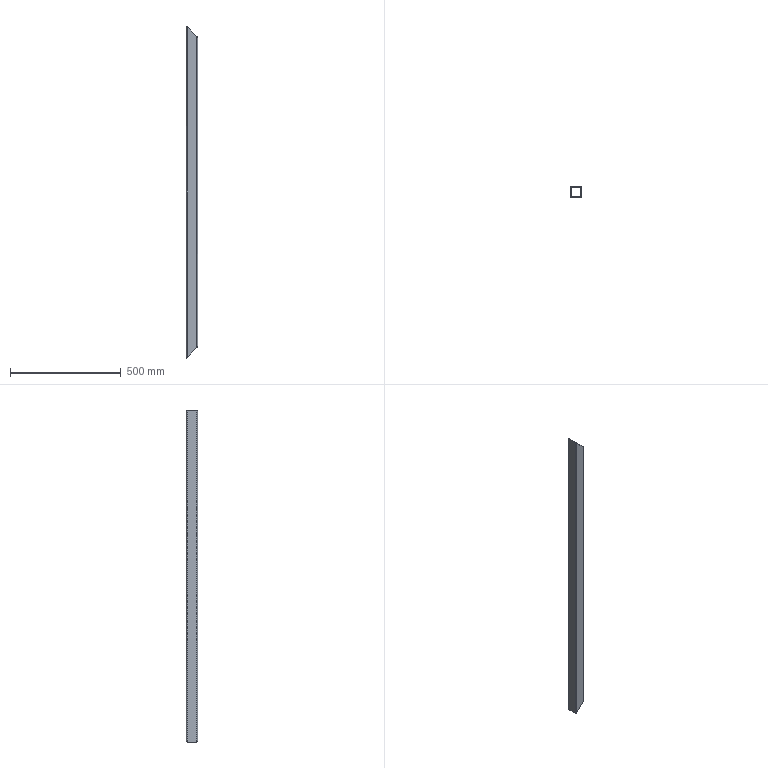Part | SolidWorks | features BaseBody 1 | 1 solid | 18 faces | box 50 x 50 x 1498 mm | volume 798027 mm3 | plane 10 | cylinder 8 | commonest cylinder face diameters 2 x4 8 x4
STEP:
#1=CARTESIAN_POINT('',(-25.,21.,-749.));
#2=VERTEX_POINT('',#1);
#3=CARTESIAN_POINT('',(-25.,-21.,-749.));
#4=VERTEX_POINT('',#3);
#5=CARTESIAN_POINT('',(-25.,21.,-749.));
#6=DIRECTION('',(0.,-1.,0.));
#7=VECTOR('',#6,1000.);
#8=LINE('',#5,#7);
#9=EDGE_CURVE('',#2,#4,#8,.T.);
#10=ORIENTED_EDGE('',*,*,#9,.T.);
#11=CARTESIAN_POINT('',(-25.,-21.,749.));
#12=VERTEX_POINT('',#11);
#13=CARTESIAN_POINT('',(-25.,-21.,749.));
#14=DIRECTION('',(0.,0.,-1.));
#15=VECTOR('',#14,1000.);
#16=LINE('',#13,#15);
#17=EDGE_CURVE('',#12,#4,#16,.T.);
#18=ORIENTED_EDGE('',*,*,#17,.F.);
#19=CARTESIAN_POINT('',(-25.,21.,749.));
#20=VERTEX_POINT('',#19);
#21=CARTESIAN_POINT('',(-25.,21.,749.));
#22=DIRECTION('',(0.,-1.,0.));
#23=VECTOR('',#22,1000.);
#24=LINE('',#21,#23);
#25=EDGE_CURVE('',#20,#12,#24,.T.);
#26=ORIENTED_EDGE('',*,*,#25,.F.);
#27=CARTESIAN_POINT('',(-25.,21.,749.));
#28=DIRECTION('',(0.,0.,-1.));
#29=VECTOR('',#28,1000.);
#30=LINE('',#27,#29);
#31=EDGE_CURVE('',#20,#2,#30,.T.);
#32=ORIENTED_EDGE('',*,*,#31,.T.);
#33=EDGE_LOOP('',(#10,#18,#26,#32));
#34=FACE_OUTER_BOUND('',#33,.T.);
#35=CARTESIAN_POINT('',(-25.,21.,749.));
#36=DIRECTION('',(1.,0.,0.));
#37=DIRECTION('',(0.,1.,0.));
#38=AXIS2_PLACEMENT_3D('',#35,#36,#37);
#39=PLANE('',#38);
#40=ADVANCED_FACE('',(#34),#39,.F.);
#41=CARTESIAN_POINT('',(-21.,25.,745.));
#42=VERTEX_POINT('',#41);
#43=CARTESIAN_POINT('',(-21.,25.,-745.));
#44=VERTEX_POINT('',#43);
#45=CARTESIAN_POINT('',(-21.,25.,749.));
#46=DIRECTION('',(0.,0.,-1.));
#47=VECTOR('',#46,1000.);
#48=LINE('',#45,#47);
#49=EDGE_CURVE('',#42,#44,#48,.T.);
#50=ORIENTED_EDGE('',*,*,#49,.T.);
#51=CARTESIAN_POINT('',(-21.,25.,-745.));
#52=CARTESIAN_POINT('',(-23.343,25.,-747.343));
#53=CARTESIAN_POINT('',(-25.,23.343,-749.));
#54=CARTESIAN_POINT('',(-25.,21.,-749.));
#55=(BOUNDED_CURVE()B_SPLINE_CURVE(3,(#51,#52,#53,#54),.UNSPECIFIED.,.F.,.F.)B_SPLINE_CURVE_WITH_KNOTS((4,4),(4.712,6.283),.UNSPECIFIED.)CURVE()GEOMETRIC_REPRESENTATION_ITEM()RATIONAL_B_SPLINE_CURVE((1.,0.8047,0.8047,1.))REPRESENTATION_ITEM(''));
#56=EDGE_CURVE('',#44,#2,#55,.T.);
#57=ORIENTED_EDGE('',*,*,#56,.T.);
#58=ORIENTED_EDGE('',*,*,#31,.F.);
#59=CARTESIAN_POINT('',(-25.,21.,749.));
#60=CARTESIAN_POINT('',(-25.,23.343,749.));
#61=CARTESIAN_POINT('',(-23.343,25.,747.343));
#62=CARTESIAN_POINT('',(-21.,25.,745.));
#63=(BOUNDED_CURVE()B_SPLINE_CURVE(3,(#59,#60,#61,#62),.UNSPECIFIED.,.F.,.T.)B_SPLINE_CURVE_WITH_KNOTS((4,4),(3.142,4.712),.UNSPECIFIED.)CURVE()GEOMETRIC_REPRESENTATION_ITEM()RATIONAL_B_SPLINE_CURVE((1.,0.8047,0.8047,1.))REPRESENTATION_ITEM(''));
#64=EDGE_CURVE('',#20,#42,#63,.T.);
#65=ORIENTED_EDGE('',*,*,#64,.T.);
#66=EDGE_LOOP('',(#50,#57,#58,#65));
#67=FACE_OUTER_BOUND('',#66,.T.);
#68=CARTESIAN_POINT('',(-21.,21.,749.));
#69=DIRECTION('',(0.,0.,-1.));
#70=DIRECTION('',(-1.,0.,0.));
#71=AXIS2_PLACEMENT_3D('',#68,#69,#70);
#72=CYLINDRICAL_SURFACE('',#71,4.);
#73=ADVANCED_FACE('',(#67),#72,.T.);
#74=CARTESIAN_POINT('',(21.,25.,703.));
#75=VERTEX_POINT('',#74);
#76=CARTESIAN_POINT('',(21.,25.,-703.));
#77=VERTEX_POINT('',#76);
#78=CARTESIAN_POINT('',(21.,25.,749.));
#79=DIRECTION('',(0.,0.,-1.));
#80=VECTOR('',#79,1000.);
#81=LINE('',#78,#80);
#82=EDGE_CURVE('',#75,#77,#81,.T.);
#83=ORIENTED_EDGE('',*,*,#82,.T.);
#84=CARTESIAN_POINT('',(-25.,25.,-749.));
#85=DIRECTION('',(0.7071,0.,0.7071));
#86=VECTOR('',#85,1000.);
#87=LINE('',#84,#86);
#88=EDGE_CURVE('',#44,#77,#87,.T.);
#89=ORIENTED_EDGE('',*,*,#88,.F.);
#90=ORIENTED_EDGE('',*,*,#49,.F.);
#91=CARTESIAN_POINT('',(-25.,25.,749.));
#92=DIRECTION('',(-0.7071,0.,0.7071));
#93=VECTOR('',#92,1000.);
#94=LINE('',#91,#93);
#95=EDGE_CURVE('',#75,#42,#94,.T.);
#96=ORIENTED_EDGE('',*,*,#95,.F.);
#97=EDGE_LOOP('',(#83,#89,#90,#96));
#98=FACE_OUTER_BOUND('',#97,.T.);
#99=CARTESIAN_POINT('',(-21.,25.,749.));
#100=DIRECTION('',(0.,-1.,0.));
#101=DIRECTION('',(0.,0.,-1.));
#102=AXIS2_PLACEMENT_3D('',#99,#100,#101);
#103=PLANE('',#102);
#104=ADVANCED_FACE('',(#98),#103,.F.);
#105=CARTESIAN_POINT('',(25.,21.,699.));
#106=VERTEX_POINT('',#105);
#107=CARTESIAN_POINT('',(25.,21.,-699.));
#108=VERTEX_POINT('',#107);
#109=CARTESIAN_POINT('',(25.,21.,749.));
#110=DIRECTION('',(0.,0.,-1.));
#111=VECTOR('',#110,1000.);
#112=LINE('',#109,#111);
#113=EDGE_CURVE('',#106,#108,#112,.T.);
#114=ORIENTED_EDGE('',*,*,#113,.T.);
#115=CARTESIAN_POINT('',(25.,21.,-699.));
#116=CARTESIAN_POINT('',(25.,23.343,-699.));
#117=CARTESIAN_POINT('',(23.343,25.,-700.657));
#118=CARTESIAN_POINT('',(21.,25.,-703.));
#119=(BOUNDED_CURVE()B_SPLINE_CURVE(3,(#115,#116,#117,#118),.UNSPECIFIED.,.F.,.F.)B_SPLINE_CURVE_WITH_KNOTS((4,4),(3.142,4.712),.UNSPECIFIED.)CURVE()GEOMETRIC_REPRESENTATION_ITEM()RATIONAL_B_SPLINE_CURVE((1.,0.8047,0.8047,1.))REPRESENTATION_ITEM(''));
#120=EDGE_CURVE('',#108,#77,#119,.T.);
#121=ORIENTED_EDGE('',*,*,#120,.T.);
#122=ORIENTED_EDGE('',*,*,#82,.F.);
#123=CARTESIAN_POINT('',(21.,25.,703.));
#124=CARTESIAN_POINT('',(23.343,25.,700.657));
#125=CARTESIAN_POINT('',(25.,23.343,699.));
#126=CARTESIAN_POINT('',(25.,21.,699.));
#127=(BOUNDED_CURVE()B_SPLINE_CURVE(3,(#123,#124,#125,#126),.UNSPECIFIED.,.F.,.F.)B_SPLINE_CURVE_WITH_KNOTS((4,4),(4.712,6.283),.UNSPECIFIED.)CURVE()GEOMETRIC_REPRESENTATION_ITEM()RATIONAL_B_SPLINE_CURVE((1.,0.8047,0.8047,1.))REPRESENTATION_ITEM(''));
#128=EDGE_CURVE('',#75,#106,#127,.T.);
#129=ORIENTED_EDGE('',*,*,#128,.T.);
#130=EDGE_LOOP('',(#114,#121,#122,#129));
#131=FACE_OUTER_BOUND('',#130,.T.);
#132=CARTESIAN_POINT('',(21.,21.,749.));
#133=DIRECTION('',(0.,0.,-1.));
#134=DIRECTION('',(-1.,0.,0.));
#135=AXIS2_PLACEMENT_3D('',#132,#133,#134);
#136=CYLINDRICAL_SURFACE('',#135,4.);
#137=ADVANCED_FACE('',(#131),#136,.T.);
#138=CARTESIAN_POINT('',(25.,-21.,699.));
#139=VERTEX_POINT('',#138);
#140=CARTESIAN_POINT('',(25.,-21.,-699.));
#141=VERTEX_POINT('',#140);
#142=CARTESIAN_POINT('',(25.,-21.,749.));
#143=DIRECTION('',(0.,0.,-1.));
#144=VECTOR('',#143,1000.);
#145=LINE('',#142,#144);
#146=EDGE_CURVE('',#139,#141,#145,.T.);
#147=ORIENTED_EDGE('',*,*,#146,.T.);
#148=CARTESIAN_POINT('',(25.,-25.,-699.));
#149=DIRECTION('',(0.,1.,0.));
#150=VECTOR('',#149,1000.);
#151=LINE('',#148,#150);
#152=EDGE_CURVE('',#141,#108,#151,.T.);
#153=ORIENTED_EDGE('',*,*,#152,.T.);
#154=ORIENTED_EDGE('',*,*,#113,.F.);
#155=CARTESIAN_POINT('',(25.,-25.,699.));
#156=DIRECTION('',(0.,1.,0.));
#157=VECTOR('',#156,1000.);
#158=LINE('',#155,#157);
#159=EDGE_CURVE('',#139,#106,#158,.T.);
#160=ORIENTED_EDGE('',*,*,#159,.F.);
#161=EDGE_LOOP('',(#147,#153,#154,#160));
#162=FACE_OUTER_BOUND('',#161,.T.);
#163=CARTESIAN_POINT('',(25.,21.,749.));
#164=DIRECTION('',(-1.,0.,0.));
#165=DIRECTION('',(0.,1.,0.));
#166=AXIS2_PLACEMENT_3D('',#163,#164,#165);
#167=PLANE('',#166);
#168=ADVANCED_FACE('',(#162),#167,.F.);
#169=CARTESIAN_POINT('',(21.,-25.,703.));
#170=VERTEX_POINT('',#169);
#171=CARTESIAN_POINT('',(21.,-25.,-703.));
#172=VERTEX_POINT('',#171);
#173=CARTESIAN_POINT('',(21.,-25.,749.));
#174=DIRECTION('',(0.,0.,-1.));
#175=VECTOR('',#174,1000.);
#176=LINE('',#173,#175);
#177=EDGE_CURVE('',#170,#172,#176,.T.);
#178=ORIENTED_EDGE('',*,*,#177,.T.);
#179=CARTESIAN_POINT('',(21.,-25.,-703.));
#180=CARTESIAN_POINT('',(23.343,-25.,-700.657));
#181=CARTESIAN_POINT('',(25.,-23.343,-699.));
#182=CARTESIAN_POINT('',(25.,-21.,-699.));
#183=(BOUNDED_CURVE()B_SPLINE_CURVE(3,(#179,#180,#181,#182),.UNSPECIFIED.,.F.,.F.)B_SPLINE_CURVE_WITH_KNOTS((4,4),(1.571,3.142),.UNSPECIFIED.)CURVE()GEOMETRIC_REPRESENTATION_ITEM()RATIONAL_B_SPLINE_CURVE((1.,0.8047,0.8047,1.))REPRESENTATION_ITEM(''));
#184=EDGE_CURVE('',#172,#141,#183,.T.);
#185=ORIENTED_EDGE('',*,*,#184,.T.);
#186=ORIENTED_EDGE('',*,*,#146,.F.);
#187=CARTESIAN_POINT('',(25.,-21.,699.));
#188=CARTESIAN_POINT('',(25.,-23.343,699.));
#189=CARTESIAN_POINT('',(23.343,-25.,700.657));
#190=CARTESIAN_POINT('',(21.,-25.,703.));
#191=(BOUNDED_CURVE()B_SPLINE_CURVE(3,(#187,#188,#189,#190),.UNSPECIFIED.,.F.,.F.)B_SPLINE_CURVE_WITH_KNOTS((4,4),(0.,1.571),.UNSPECIFIED.)CURVE()GEOMETRIC_REPRESENTATION_ITEM()RATIONAL_B_SPLINE_CURVE((1.,0.8047,0.8047,1.))REPRESENTATION_ITEM(''));
#192=EDGE_CURVE('',#139,#170,#191,.T.);
#193=ORIENTED_EDGE('',*,*,#192,.T.);
#194=EDGE_LOOP('',(#178,#185,#186,#193));
#195=FACE_OUTER_BOUND('',#194,.T.);
#196=CARTESIAN_POINT('',(21.,-21.,749.));
#197=DIRECTION('',(0.,0.,-1.));
#198=DIRECTION('',(-1.,0.,0.));
#199=AXIS2_PLACEMENT_3D('',#196,#197,#198);
#200=CYLINDRICAL_SURFACE('',#199,4.);
#201=ADVANCED_FACE('',(#195),#200,.T.);
#202=CARTESIAN_POINT('',(-21.,-25.,745.));
#203=VERTEX_POINT('',#202);
#204=CARTESIAN_POINT('',(-21.,-25.,-745.));
#205=VERTEX_POINT('',#204);
#206=CARTESIAN_POINT('',(-21.,-25.,749.));
#207=DIRECTION('',(0.,0.,-1.));
#208=VECTOR('',#207,1000.);
#209=LINE('',#206,#208);
#210=EDGE_CURVE('',#203,#205,#209,.T.);
#211=ORIENTED_EDGE('',*,*,#210,.T.);
#212=CARTESIAN_POINT('',(-25.,-25.,-749.));
#213=DIRECTION('',(0.7071,0.,0.7071));
#214=VECTOR('',#213,1000.);
#215=LINE('',#212,#214);
#216=EDGE_CURVE('',#205,#172,#215,.T.);
#217=ORIENTED_EDGE('',*,*,#216,.T.);
#218=ORIENTED_EDGE('',*,*,#177,.F.);
#219=CARTESIAN_POINT('',(-25.,-25.,749.));
#220=DIRECTION('',(-0.7071,0.,0.7071));
#221=VECTOR('',#220,1000.);
#222=LINE('',#219,#221);
#223=EDGE_CURVE('',#170,#203,#222,.T.);
#224=ORIENTED_EDGE('',*,*,#223,.T.);
#225=EDGE_LOOP('',(#211,#217,#218,#224));
#226=FACE_OUTER_BOUND('',#225,.T.);
#227=CARTESIAN_POINT('',(-21.,-25.,749.));
#228=DIRECTION('',(0.,1.,0.));
#229=DIRECTION('',(1.,0.,0.));
#230=AXIS2_PLACEMENT_3D('',#227,#228,#229);
#231=PLANE('',#230);
#232=ADVANCED_FACE('',(#226),#231,.F.);
#233=ORIENTED_EDGE('',*,*,#17,.T.);
#234=CARTESIAN_POINT('',(-25.,-21.,-749.));
#235=CARTESIAN_POINT('',(-25.,-23.343,-749.));
#236=CARTESIAN_POINT('',(-23.343,-25.,-747.343));
#237=CARTESIAN_POINT('',(-21.,-25.,-745.));
#238=(BOUNDED_CURVE()B_SPLINE_CURVE(3,(#234,#235,#236,#237),.UNSPECIFIED.,.F.,.F.)B_SPLINE_CURVE_WITH_KNOTS((4,4),(0.,1.571),.UNSPECIFIED.)CURVE()GEOMETRIC_REPRESENTATION_ITEM()RATIONAL_B_SPLINE_CURVE((1.,0.8047,0.8047,1.))REPRESENTATION_ITEM(''));
#239=EDGE_CURVE('',#4,#205,#238,.T.);
#240=ORIENTED_EDGE('',*,*,#239,.T.);
#241=ORIENTED_EDGE('',*,*,#210,.F.);
#242=CARTESIAN_POINT('',(-21.,-25.,745.));
#243=CARTESIAN_POINT('',(-23.343,-25.,747.343));
#244=CARTESIAN_POINT('',(-25.,-23.343,749.));
#245=CARTESIAN_POINT('',(-25.,-21.,749.));
#246=(BOUNDED_CURVE()B_SPLINE_CURVE(3,(#242,#243,#244,#245),.UNSPECIFIED.,.F.,.F.)B_SPLINE_CURVE_WITH_KNOTS((4,4),(1.571,3.142),.UNSPECIFIED.)CURVE()GEOMETRIC_REPRESENTATION_ITEM()RATIONAL_B_SPLINE_CURVE((1.,0.8047,0.8047,1.))REPRESENTATION_ITEM(''));
#247=EDGE_CURVE('',#203,#12,#246,.T.);
#248=ORIENTED_EDGE('',*,*,#247,.T.);
#249=EDGE_LOOP('',(#233,#240,#241,#248));
#250=FACE_OUTER_BOUND('',#249,.T.);
#251=CARTESIAN_POINT('',(-21.,-21.,749.));
#252=DIRECTION('',(0.,0.,-1.));
#253=DIRECTION('',(-1.,0.,0.));
#254=AXIS2_PLACEMENT_3D('',#251,#252,#253);
#255=CYLINDRICAL_SURFACE('',#254,4.);
#256=ADVANCED_FACE('',(#250),#255,.T.);
#257=CARTESIAN_POINT('',(-22.,-21.,-746.));
#258=VERTEX_POINT('',#257);
#259=CARTESIAN_POINT('',(-21.,-22.,-745.));
#260=VERTEX_POINT('',#259);
#261=CARTESIAN_POINT('',(-22.,-21.,-746.));
#262=CARTESIAN_POINT('',(-22.,-21.586,-746.));
#263=CARTESIAN_POINT('',(-21.586,-22.,-745.586));
#264=CARTESIAN_POINT('',(-21.,-22.,-745.));
#265=(BOUNDED_CURVE()B_SPLINE_CURVE(3,(#261,#262,#263,#264),.UNSPECIFIED.,.F.,.F.)B_SPLINE_CURVE_WITH_KNOTS((4,4),(0.,1.571),.UNSPECIFIED.)CURVE()GEOMETRIC_REPRESENTATION_ITEM()RATIONAL_B_SPLINE_CURVE((1.,0.8047,0.8047,1.))REPRESENTATION_ITEM(''));
#266=EDGE_CURVE('',#258,#260,#265,.T.);
#267=ORIENTED_EDGE('',*,*,#266,.T.);
#268=CARTESIAN_POINT('',(21.,-22.,-703.));
#269=VERTEX_POINT('',#268);
#270=CARTESIAN_POINT('',(726.,-22.,2.));
#271=DIRECTION('',(0.7071,0.,0.7071));
#272=VECTOR('',#271,1000.);
#273=LINE('',#270,#272);
#274=EDGE_CURVE('',#260,#269,#273,.T.);
#275=ORIENTED_EDGE('',*,*,#274,.T.);
#276=CARTESIAN_POINT('',(22.,-21.,-702.));
#277=VERTEX_POINT('',#276);
#278=CARTESIAN_POINT('',(21.,-22.,-703.));
#279=CARTESIAN_POINT('',(21.586,-22.,-702.414));
#280=CARTESIAN_POINT('',(22.,-21.586,-702.));
#281=CARTESIAN_POINT('',(22.,-21.,-702.));
#282=(BOUNDED_CURVE()B_SPLINE_CURVE(3,(#278,#279,#280,#281),.UNSPECIFIED.,.F.,.F.)B_SPLINE_CURVE_WITH_KNOTS((4,4),(1.571,3.142),.UNSPECIFIED.)CURVE()GEOMETRIC_REPRESENTATION_ITEM()RATIONAL_B_SPLINE_CURVE((1.,0.8047,0.8047,1.))REPRESENTATION_ITEM(''));
#283=EDGE_CURVE('',#269,#277,#282,.T.);
#284=ORIENTED_EDGE('',*,*,#283,.T.);
#285=CARTESIAN_POINT('',(22.,21.,-702.));
#286=VERTEX_POINT('',#285);
#287=CARTESIAN_POINT('',(22.,21.,-702.));
#288=DIRECTION('',(0.,1.,0.));
#289=VECTOR('',#288,1000.);
#290=LINE('',#287,#289);
#291=EDGE_CURVE('',#277,#286,#290,.T.);
#292=ORIENTED_EDGE('',*,*,#291,.T.);
#293=CARTESIAN_POINT('',(21.,22.,-703.));
#294=VERTEX_POINT('',#293);
#295=CARTESIAN_POINT('',(22.,21.,-702.));
#296=CARTESIAN_POINT('',(22.,21.586,-702.));
#297=CARTESIAN_POINT('',(21.586,22.,-702.414));
#298=CARTESIAN_POINT('',(21.,22.,-703.));
#299=(BOUNDED_CURVE()B_SPLINE_CURVE(3,(#295,#296,#297,#298),.UNSPECIFIED.,.F.,.F.)B_SPLINE_CURVE_WITH_KNOTS((4,4),(3.142,4.712),.UNSPECIFIED.)CURVE()GEOMETRIC_REPRESENTATION_ITEM()RATIONAL_B_SPLINE_CURVE((1.,0.8047,0.8047,1.))REPRESENTATION_ITEM(''));
#300=EDGE_CURVE('',#286,#294,#299,.T.);
#301=ORIENTED_EDGE('',*,*,#300,.T.);
#302=CARTESIAN_POINT('',(-21.,22.,-745.));
#303=VERTEX_POINT('',#302);
#304=CARTESIAN_POINT('',(726.,22.,2.));
#305=DIRECTION('',(-0.7071,0.,-0.7071));
#306=VECTOR('',#305,1000.);
#307=LINE('',#304,#306);
#308=EDGE_CURVE('',#294,#303,#307,.T.);
#309=ORIENTED_EDGE('',*,*,#308,.T.);
#310=CARTESIAN_POINT('',(-22.,21.,-746.));
#311=VERTEX_POINT('',#310);
#312=CARTESIAN_POINT('',(-21.,22.,-745.));
#313=CARTESIAN_POINT('',(-21.586,22.,-745.586));
#314=CARTESIAN_POINT('',(-22.,21.586,-746.));
#315=CARTESIAN_POINT('',(-22.,21.,-746.));
#316=(BOUNDED_CURVE()B_SPLINE_CURVE(3,(#312,#313,#314,#315),.UNSPECIFIED.,.F.,.F.)B_SPLINE_CURVE_WITH_KNOTS((4,4),(4.712,6.283),.UNSPECIFIED.)CURVE()GEOMETRIC_REPRESENTATION_ITEM()RATIONAL_B_SPLINE_CURVE((1.,0.8047,0.8047,1.))REPRESENTATION_ITEM(''));
#317=EDGE_CURVE('',#303,#311,#316,.T.);
#318=ORIENTED_EDGE('',*,*,#317,.T.);
#319=CARTESIAN_POINT('',(-22.,21.,-746.));
#320=DIRECTION('',(0.,-1.,0.));
#321=VECTOR('',#320,1000.);
#322=LINE('',#319,#321);
#323=EDGE_CURVE('',#311,#258,#322,.T.);
#324=ORIENTED_EDGE('',*,*,#323,.T.);
#325=EDGE_LOOP('',(#267,#275,#284,#292,#301,#309,#318,#324));
#326=FACE_BOUND('',#325,.T.);
#327=ORIENTED_EDGE('',*,*,#9,.F.);
#328=ORIENTED_EDGE('',*,*,#56,.F.);
#329=ORIENTED_EDGE('',*,*,#88,.T.);
#330=ORIENTED_EDGE('',*,*,#120,.F.);
#331=ORIENTED_EDGE('',*,*,#152,.F.);
#332=ORIENTED_EDGE('',*,*,#184,.F.);
#333=ORIENTED_EDGE('',*,*,#216,.F.);
#334=ORIENTED_EDGE('',*,*,#239,.F.);
#335=EDGE_LOOP('',(#327,#328,#329,#330,#331,#332,#333,#334));
#336=FACE_OUTER_BOUND('',#335,.T.);
#337=CARTESIAN_POINT('',(-25.,-25.,-749.));
#338=DIRECTION('',(-0.7071,0.,0.7071));
#339=DIRECTION('',(0.,1.,0.));
#340=AXIS2_PLACEMENT_3D('',#337,#338,#339);
#341=PLANE('',#340);
#342=ADVANCED_FACE('',(#326,#336),#341,.F.);
#343=CARTESIAN_POINT('',(-21.,-22.,745.));
#344=VERTEX_POINT('',#343);
#345=CARTESIAN_POINT('',(-22.,-21.,746.));
#346=VERTEX_POINT('',#345);
#347=CARTESIAN_POINT('',(-21.,-22.,745.));
#348=CARTESIAN_POINT('',(-21.586,-22.,745.586));
#349=CARTESIAN_POINT('',(-22.,-21.586,746.));
#350=CARTESIAN_POINT('',(-22.,-21.,746.));
#351=(BOUNDED_CURVE()B_SPLINE_CURVE(3,(#347,#348,#349,#350),.UNSPECIFIED.,.F.,.F.)B_SPLINE_CURVE_WITH_KNOTS((4,4),(1.571,3.142),.UNSPECIFIED.)CURVE()GEOMETRIC_REPRESENTATION_ITEM()RATIONAL_B_SPLINE_CURVE((1.,0.8047,0.8047,1.))REPRESENTATION_ITEM(''));
#352=EDGE_CURVE('',#344,#346,#351,.T.);
#353=ORIENTED_EDGE('',*,*,#352,.T.);
#354=CARTESIAN_POINT('',(-22.,21.,746.));
#355=VERTEX_POINT('',#354);
#356=CARTESIAN_POINT('',(-22.,21.,746.));
#357=DIRECTION('',(0.,1.,0.));
#358=VECTOR('',#357,1000.);
#359=LINE('',#356,#358);
#360=EDGE_CURVE('',#346,#355,#359,.T.);
#361=ORIENTED_EDGE('',*,*,#360,.T.);
#362=CARTESIAN_POINT('',(-21.,22.,745.));
#363=VERTEX_POINT('',#362);
#364=CARTESIAN_POINT('',(-22.,21.,746.));
#365=CARTESIAN_POINT('',(-22.,21.586,746.));
#366=CARTESIAN_POINT('',(-21.586,22.,745.586));
#367=CARTESIAN_POINT('',(-21.,22.,745.));
#368=(BOUNDED_CURVE()B_SPLINE_CURVE(3,(#364,#365,#366,#367),.UNSPECIFIED.,.F.,.F.)B_SPLINE_CURVE_WITH_KNOTS((4,4),(3.142,4.712),.UNSPECIFIED.)CURVE()GEOMETRIC_REPRESENTATION_ITEM()RATIONAL_B_SPLINE_CURVE((1.,0.8047,0.8047,1.))REPRESENTATION_ITEM(''));
#369=EDGE_CURVE('',#355,#363,#368,.T.);
#370=ORIENTED_EDGE('',*,*,#369,.T.);
#371=CARTESIAN_POINT('',(21.,22.,703.));
#372=VERTEX_POINT('',#371);
#373=CARTESIAN_POINT('',(-23.,22.,747.));
#374=DIRECTION('',(0.7071,0.,-0.7071));
#375=VECTOR('',#374,1000.);
#376=LINE('',#373,#375);
#377=EDGE_CURVE('',#363,#372,#376,.T.);
#378=ORIENTED_EDGE('',*,*,#377,.T.);
#379=CARTESIAN_POINT('',(22.,21.,702.));
#380=VERTEX_POINT('',#379);
#381=CARTESIAN_POINT('',(21.,22.,703.));
#382=CARTESIAN_POINT('',(21.586,22.,702.414));
#383=CARTESIAN_POINT('',(22.,21.586,702.));
#384=CARTESIAN_POINT('',(22.,21.,702.));
#385=(BOUNDED_CURVE()B_SPLINE_CURVE(3,(#381,#382,#383,#384),.UNSPECIFIED.,.F.,.F.)B_SPLINE_CURVE_WITH_KNOTS((4,4),(4.712,6.283),.UNSPECIFIED.)CURVE()GEOMETRIC_REPRESENTATION_ITEM()RATIONAL_B_SPLINE_CURVE((1.,0.8047,0.8047,1.))REPRESENTATION_ITEM(''));
#386=EDGE_CURVE('',#372,#380,#385,.T.);
#387=ORIENTED_EDGE('',*,*,#386,.T.);
#388=CARTESIAN_POINT('',(22.,-21.,702.));
#389=VERTEX_POINT('',#388);
#390=CARTESIAN_POINT('',(22.,21.,702.));
#391=DIRECTION('',(0.,-1.,0.));
#392=VECTOR('',#391,1000.);
#393=LINE('',#390,#392);
#394=EDGE_CURVE('',#380,#389,#393,.T.);
#395=ORIENTED_EDGE('',*,*,#394,.T.);
#396=CARTESIAN_POINT('',(21.,-22.,703.));
#397=VERTEX_POINT('',#396);
#398=CARTESIAN_POINT('',(22.,-21.,702.));
#399=CARTESIAN_POINT('',(22.,-21.586,702.));
#400=CARTESIAN_POINT('',(21.586,-22.,702.414));
#401=CARTESIAN_POINT('',(21.,-22.,703.));
#402=(BOUNDED_CURVE()B_SPLINE_CURVE(3,(#398,#399,#400,#401),.UNSPECIFIED.,.F.,.F.)B_SPLINE_CURVE_WITH_KNOTS((4,4),(0.,1.571),.UNSPECIFIED.)CURVE()GEOMETRIC_REPRESENTATION_ITEM()RATIONAL_B_SPLINE_CURVE((1.,0.8047,0.8047,1.))REPRESENTATION_ITEM(''));
#403=EDGE_CURVE('',#389,#397,#402,.T.);
#404=ORIENTED_EDGE('',*,*,#403,.T.);
#405=CARTESIAN_POINT('',(-23.,-22.,747.));
#406=DIRECTION('',(-0.7071,0.,0.7071));
#407=VECTOR('',#406,1000.);
#408=LINE('',#405,#407);
#409=EDGE_CURVE('',#397,#344,#408,.T.);
#410=ORIENTED_EDGE('',*,*,#409,.T.);
#411=EDGE_LOOP('',(#353,#361,#370,#378,#387,#395,#404,#410));
#412=FACE_BOUND('',#411,.T.);
#413=ORIENTED_EDGE('',*,*,#223,.F.);
#414=ORIENTED_EDGE('',*,*,#192,.F.);
#415=ORIENTED_EDGE('',*,*,#159,.T.);
#416=ORIENTED_EDGE('',*,*,#128,.F.);
#417=ORIENTED_EDGE('',*,*,#95,.T.);
#418=ORIENTED_EDGE('',*,*,#64,.F.);
#419=ORIENTED_EDGE('',*,*,#25,.T.);
#420=ORIENTED_EDGE('',*,*,#247,.F.);
#421=EDGE_LOOP('',(#413,#414,#415,#416,#417,#418,#419,#420));
#422=FACE_OUTER_BOUND('',#421,.T.);
#423=CARTESIAN_POINT('',(-25.,-25.,749.));
#424=DIRECTION('',(-0.7071,0.,-0.7071));
#425=DIRECTION('',(-0.7071,0.,0.7071));
#426=AXIS2_PLACEMENT_3D('',#423,#424,#425);
#427=PLANE('',#426);
#428=ADVANCED_FACE('',(#412,#422),#427,.F.);
#429=ORIENTED_EDGE('',*,*,#266,.F.);
#430=CARTESIAN_POINT('',(-22.,-21.,749.));
#431=DIRECTION('',(0.,0.,-1.));
#432=VECTOR('',#431,1000.);
#433=LINE('',#430,#432);
#434=EDGE_CURVE('',#346,#258,#433,.T.);
#435=ORIENTED_EDGE('',*,*,#434,.F.);
#436=ORIENTED_EDGE('',*,*,#352,.F.);
#437=CARTESIAN_POINT('',(-21.,-22.,749.));
#438=DIRECTION('',(0.,0.,-1.));
#439=VECTOR('',#438,1000.);
#440=LINE('',#437,#439);
#441=EDGE_CURVE('',#344,#260,#440,.T.);
#442=ORIENTED_EDGE('',*,*,#441,.T.);
#443=EDGE_LOOP('',(#429,#435,#436,#442));
#444=FACE_OUTER_BOUND('',#443,.T.);
#445=CARTESIAN_POINT('',(-21.,-21.,749.));
#446=DIRECTION('',(0.,0.,-1.));
#447=DIRECTION('',(-1.,0.,0.));
#448=AXIS2_PLACEMENT_3D('',#445,#446,#447);
#449=CYLINDRICAL_SURFACE('',#448,1.);
#450=ADVANCED_FACE('',(#444),#449,.F.);
#451=ORIENTED_EDGE('',*,*,#274,.F.);
#452=ORIENTED_EDGE('',*,*,#441,.F.);
#453=ORIENTED_EDGE('',*,*,#409,.F.);
#454=CARTESIAN_POINT('',(21.,-22.,749.));
#455=DIRECTION('',(0.,0.,-1.));
#456=VECTOR('',#455,1000.);
#457=LINE('',#454,#456);
#458=EDGE_CURVE('',#397,#269,#457,.T.);
#459=ORIENTED_EDGE('',*,*,#458,.T.);
#460=EDGE_LOOP('',(#451,#452,#453,#459));
#461=FACE_OUTER_BOUND('',#460,.T.);
#462=CARTESIAN_POINT('',(-21.,-22.,749.));
#463=DIRECTION('',(0.,1.,0.));
#464=DIRECTION('',(1.,0.,0.));
#465=AXIS2_PLACEMENT_3D('',#462,#463,#464);
#466=PLANE('',#465);
#467=ADVANCED_FACE('',(#461),#466,.T.);
#468=ORIENTED_EDGE('',*,*,#283,.F.);
#469=ORIENTED_EDGE('',*,*,#458,.F.);
#470=ORIENTED_EDGE('',*,*,#403,.F.);
#471=CARTESIAN_POINT('',(22.,-21.,749.));
#472=DIRECTION('',(0.,0.,-1.));
#473=VECTOR('',#472,1000.);
#474=LINE('',#471,#473);
#475=EDGE_CURVE('',#389,#277,#474,.T.);
#476=ORIENTED_EDGE('',*,*,#475,.T.);
#477=EDGE_LOOP('',(#468,#469,#470,#476));
#478=FACE_OUTER_BOUND('',#477,.T.);
#479=CARTESIAN_POINT('',(21.,-21.,749.));
#480=DIRECTION('',(0.,0.,-1.));
#481=DIRECTION('',(-1.,0.,0.));
#482=AXIS2_PLACEMENT_3D('',#479,#480,#481);
#483=CYLINDRICAL_SURFACE('',#482,1.);
#484=ADVANCED_FACE('',(#478),#483,.F.);
#485=ORIENTED_EDGE('',*,*,#291,.F.);
#486=ORIENTED_EDGE('',*,*,#475,.F.);
#487=ORIENTED_EDGE('',*,*,#394,.F.);
#488=CARTESIAN_POINT('',(22.,21.,749.));
#489=DIRECTION('',(0.,0.,-1.));
#490=VECTOR('',#489,1000.);
#491=LINE('',#488,#490);
#492=EDGE_CURVE('',#380,#286,#491,.T.);
#493=ORIENTED_EDGE('',*,*,#492,.T.);
#494=EDGE_LOOP('',(#485,#486,#487,#493));
#495=FACE_OUTER_BOUND('',#494,.T.);
#496=CARTESIAN_POINT('',(22.,21.,749.));
#497=DIRECTION('',(-1.,0.,0.));
#498=DIRECTION('',(0.,1.,0.));
#499=AXIS2_PLACEMENT_3D('',#496,#497,#498);
#500=PLANE('',#499);
#501=ADVANCED_FACE('',(#495),#500,.T.);
#502=ORIENTED_EDGE('',*,*,#300,.F.);
#503=ORIENTED_EDGE('',*,*,#492,.F.);
#504=ORIENTED_EDGE('',*,*,#386,.F.);
#505=CARTESIAN_POINT('',(21.,22.,749.));
#506=DIRECTION('',(0.,0.,-1.));
#507=VECTOR('',#506,1000.);
#508=LINE('',#505,#507);
#509=EDGE_CURVE('',#372,#294,#508,.T.);
#510=ORIENTED_EDGE('',*,*,#509,.T.);
#511=EDGE_LOOP('',(#502,#503,#504,#510));
#512=FACE_OUTER_BOUND('',#511,.T.);
#513=CARTESIAN_POINT('',(21.,21.,749.));
#514=DIRECTION('',(0.,0.,-1.));
#515=DIRECTION('',(-1.,0.,0.));
#516=AXIS2_PLACEMENT_3D('',#513,#514,#515);
#517=CYLINDRICAL_SURFACE('',#516,1.);
#518=ADVANCED_FACE('',(#512),#517,.F.);
#519=ORIENTED_EDGE('',*,*,#308,.F.);
#520=ORIENTED_EDGE('',*,*,#509,.F.);
#521=ORIENTED_EDGE('',*,*,#377,.F.);
#522=CARTESIAN_POINT('',(-21.,22.,749.));
#523=DIRECTION('',(0.,0.,-1.));
#524=VECTOR('',#523,1000.);
#525=LINE('',#522,#524);
#526=EDGE_CURVE('',#363,#303,#525,.T.);
#527=ORIENTED_EDGE('',*,*,#526,.T.);
#528=EDGE_LOOP('',(#519,#520,#521,#527));
#529=FACE_OUTER_BOUND('',#528,.T.);
#530=CARTESIAN_POINT('',(-21.,22.,749.));
#531=DIRECTION('',(0.,-1.,0.));
#532=DIRECTION('',(0.,0.,-1.));
#533=AXIS2_PLACEMENT_3D('',#530,#531,#532);
#534=PLANE('',#533);
#535=ADVANCED_FACE('',(#529),#534,.T.);
#536=ORIENTED_EDGE('',*,*,#317,.F.);
#537=ORIENTED_EDGE('',*,*,#526,.F.);
#538=ORIENTED_EDGE('',*,*,#369,.F.);
#539=CARTESIAN_POINT('',(-22.,21.,749.));
#540=DIRECTION('',(0.,0.,-1.));
#541=VECTOR('',#540,1000.);
#542=LINE('',#539,#541);
#543=EDGE_CURVE('',#355,#311,#542,.T.);
#544=ORIENTED_EDGE('',*,*,#543,.T.);
#545=EDGE_LOOP('',(#536,#537,#538,#544));
#546=FACE_OUTER_BOUND('',#545,.T.);
#547=CARTESIAN_POINT('',(-21.,21.,749.));
#548=DIRECTION('',(0.,0.,-1.));
#549=DIRECTION('',(-1.,0.,0.));
#550=AXIS2_PLACEMENT_3D('',#547,#548,#549);
#551=CYLINDRICAL_SURFACE('',#550,1.);
#552=ADVANCED_FACE('',(#546),#551,.F.);
#553=ORIENTED_EDGE('',*,*,#323,.F.);
#554=ORIENTED_EDGE('',*,*,#543,.F.);
#555=ORIENTED_EDGE('',*,*,#360,.F.);
#556=ORIENTED_EDGE('',*,*,#434,.T.);
#557=EDGE_LOOP('',(#553,#554,#555,#556));
#558=FACE_OUTER_BOUND('',#557,.T.);
#559=CARTESIAN_POINT('',(-22.,21.,749.));
#560=DIRECTION('',(1.,0.,0.));
#561=DIRECTION('',(0.,1.,0.));
#562=AXIS2_PLACEMENT_3D('',#559,#560,#561);
#563=PLANE('',#562);
#564=ADVANCED_FACE('',(#558),#563,.T.);
#565=CLOSED_SHELL('',(#40,#73,#104,#137,#168,#201,#232,#256,#342,#428,#450,#467,#484,#501,#518,#535,#552,#564));
#566=MANIFOLD_SOLID_BREP('',#565);
#567=CARTESIAN_POINT('',(0.,0.,0.));
#568=DIRECTION('',(0.,0.,1.));
#569=DIRECTION('',(1.,0.,0.));
#570=AXIS2_PLACEMENT_3D('',#567,#568,#569);
#571=(LENGTH_UNIT()NAMED_UNIT(*)SI_UNIT(.MILLI.,.METRE.));
#572=UNCERTAINTY_MEASURE_WITH_UNIT(LENGTH_MEASURE(0.00001),#571,'','');
#573=(NAMED_UNIT(*)PLANE_ANGLE_UNIT()SI_UNIT($,.RADIAN.));
#574=(NAMED_UNIT(*)SI_UNIT($,.STERADIAN.)SOLID_ANGLE_UNIT());
#575=(GEOMETRIC_REPRESENTATION_CONTEXT(3)GLOBAL_UNCERTAINTY_ASSIGNED_CONTEXT((#572))GLOBAL_UNIT_ASSIGNED_CONTEXT((#571,#573,#574))REPRESENTATION_CONTEXT('',''));
#576=ADVANCED_BREP_SHAPE_REPRESENTATION('',(#566,#570),#575);